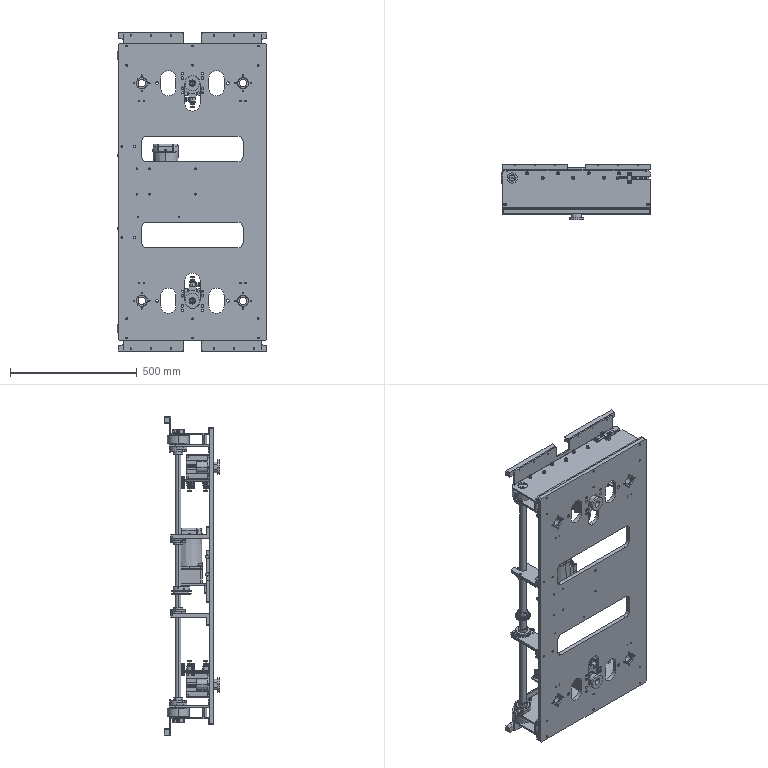Part | SolidWorks | 169 solids | 11791 faces | volume 18460750 mm3 | cylinder 4256 | plane 4120 | spline 2352 | cone 993 | torus 54 | sphere 16 | commonest cylinder face diameters 12 x394 30.636 x288 0.2 x212 8.51 x184 10 x160 76.481 x136